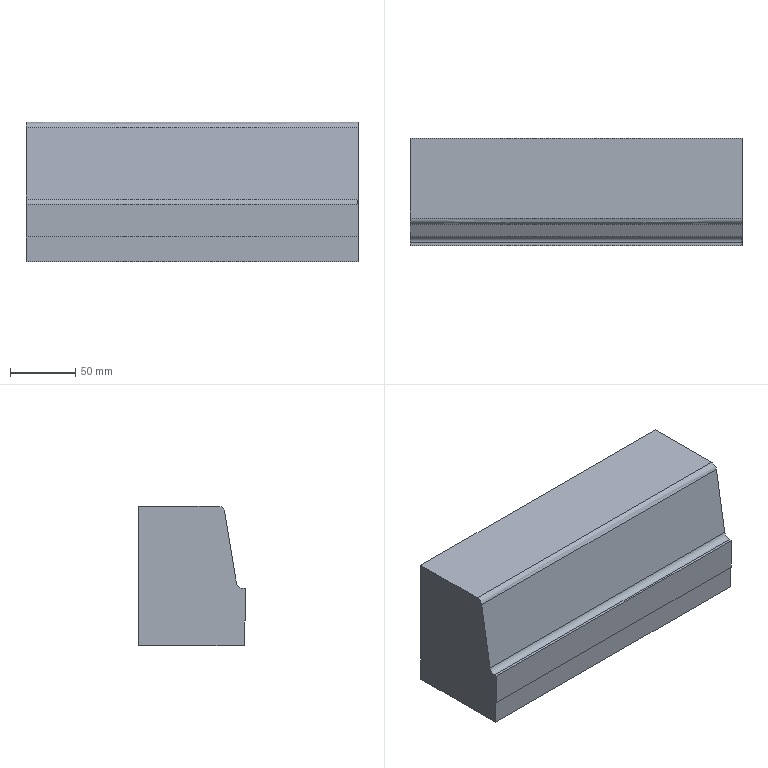Part | NX | features solid 2 | 1 solid | 22 faces | box 255 x 82.128 x 107.133 mm | volume 2023073 mm3 | plane 9 | cylinder 6 | spline 4 | cone 3 | commonest cylinder face diameters 12 x3 20 x2 10 x1
STEP:
#1=CARTESIAN_POINT('',(150.,175.,-20.));
#2=VERTEX_POINT('',#1);
#3=CARTESIAN_POINT('',(150.,175.,-30.));
#4=DIRECTION('',(0.,1.,0.));
#5=DIRECTION('',(0.,0.,1.));
#6=AXIS2_PLACEMENT_3D('',#3,#4,#5);
#7=CIRCLE('',#6,10.);
#8=EDGE_CURVE('',#2,#2,#7,.F.);
#9=ORIENTED_EDGE('',*,*,#8,.T.);
#10=EDGE_LOOP('',(#9));
#11=FACE_BOUND('',#10,.T.);
#12=CARTESIAN_POINT('',(-25.,175.,-20.));
#13=VERTEX_POINT('',#12);
#14=CARTESIAN_POINT('',(-25.,175.,-30.));
#15=DIRECTION('',(0.,1.,0.));
#16=DIRECTION('',(0.,0.,1.));
#17=AXIS2_PLACEMENT_3D('',#14,#15,#16);
#18=CIRCLE('',#17,10.);
#19=EDGE_CURVE('',#13,#13,#18,.F.);
#20=ORIENTED_EDGE('',*,*,#19,.T.);
#21=EDGE_LOOP('',(#20));
#22=FACE_BOUND('',#21,.T.);
#23=CARTESIAN_POINT('',(165.,175.,1.));
#24=VERTEX_POINT('',#23);
#25=CARTESIAN_POINT('',(165.,175.,-5.));
#26=DIRECTION('',(0.,1.,0.));
#27=DIRECTION('',(0.,0.,1.));
#28=AXIS2_PLACEMENT_3D('',#25,#26,#27);
#29=CIRCLE('',#28,6.);
#30=EDGE_CURVE('',#24,#24,#29,.F.);
#31=ORIENTED_EDGE('',*,*,#30,.T.);
#32=EDGE_LOOP('',(#31));
#33=FACE_BOUND('',#32,.T.);
#34=CARTESIAN_POINT('',(65.,175.,-24.));
#35=VERTEX_POINT('',#34);
#36=CARTESIAN_POINT('',(65.,175.,-30.));
#37=DIRECTION('',(0.,1.,0.));
#38=DIRECTION('',(0.,0.,1.));
#39=AXIS2_PLACEMENT_3D('',#36,#37,#38);
#40=CIRCLE('',#39,6.);
#41=EDGE_CURVE('',#35,#35,#40,.F.);
#42=ORIENTED_EDGE('',*,*,#41,.T.);
#43=EDGE_LOOP('',(#42));
#44=FACE_BOUND('',#43,.T.);
#45=CARTESIAN_POINT('',(-40.,175.,1.));
#46=VERTEX_POINT('',#45);
#47=CARTESIAN_POINT('',(-40.,175.,-5.));
#48=DIRECTION('',(0.,1.,0.));
#49=DIRECTION('',(0.,0.,1.));
#50=AXIS2_PLACEMENT_3D('',#47,#48,#49);
#51=CIRCLE('',#50,6.);
#52=EDGE_CURVE('',#46,#46,#51,.F.);
#53=ORIENTED_EDGE('',*,*,#52,.T.);
#54=EDGE_LOOP('',(#53));
#55=FACE_BOUND('',#54,.T.);
#56=CARTESIAN_POINT('',(190.,175.,57.133));
#57=VERTEX_POINT('',#56);
#58=CARTESIAN_POINT('',(190.,175.,-50.));
#59=VERTEX_POINT('',#58);
#60=CARTESIAN_POINT('',(190.,175.,-10.));
#61=DIRECTION('',(0.,0.,-1.));
#62=VECTOR('',#61,1000.);
#63=LINE('',#60,#62);
#64=EDGE_CURVE('',#57,#59,#63,.T.);
#65=ORIENTED_EDGE('',*,*,#64,.T.);
#66=CARTESIAN_POINT('',(-65.,175.,-50.));
#67=VERTEX_POINT('',#66);
#68=CARTESIAN_POINT('',(695.224,175.,-50.));
#69=DIRECTION('',(-1.,0.,0.));
#70=VECTOR('',#69,1000.);
#71=LINE('',#68,#70);
#72=EDGE_CURVE('',#59,#67,#71,.T.);
#73=ORIENTED_EDGE('',*,*,#72,.T.);
#74=CARTESIAN_POINT('',(-65.,175.,57.133));
#75=VERTEX_POINT('',#74);
#76=CARTESIAN_POINT('',(-65.,175.,0.));
#77=DIRECTION('',(0.,0.,1.));
#78=VECTOR('',#77,1000.);
#79=LINE('',#76,#78);
#80=EDGE_CURVE('',#67,#75,#79,.T.);
#81=ORIENTED_EDGE('',*,*,#80,.T.);
#82=CARTESIAN_POINT('',(750.,175.,57.133));
#83=DIRECTION('',(-1.,0.,0.));
#84=VECTOR('',#83,1000.);
#85=LINE('',#82,#84);
#86=EDGE_CURVE('',#57,#75,#85,.T.);
#87=ORIENTED_EDGE('',*,*,#86,.F.);
#88=EDGE_LOOP('',(#65,#73,#81,#87));
#89=FACE_BOUND('',#88,.T.);
#90=CARTESIAN_POINT('',(750.,175.,-10.));
#91=DIRECTION('',(0.,1.,0.));
#92=DIRECTION('',(0.,0.,1.));
#93=AXIS2_PLACEMENT_3D('',#90,#91,#92);
#94=PLANE('',#93);
#95=ADVANCED_FACE('',(#11,#22,#33,#44,#55,#89),#94,.T.);
#96=CARTESIAN_POINT('',(190.,108.917,52.95));
#97=VERTEX_POINT('',#96);
#98=CARTESIAN_POINT('',(-65.,108.917,52.95));
#99=VERTEX_POINT('',#98);
#100=CARTESIAN_POINT('',(190.,108.917,52.95));
#101=CARTESIAN_POINT('',(105.,108.917,52.95));
#102=CARTESIAN_POINT('',(20.,108.917,52.95));
#103=CARTESIAN_POINT('',(-65.,108.917,52.95));
#104=B_SPLINE_CURVE_WITH_KNOTS('',3,(#100,#101,#102,#103),.UNSPECIFIED.,.F.,.F.,(4,4),(0.1755,0.623),.UNSPECIFIED.);
#105=EDGE_CURVE('',#97,#99,#104,.T.);
#106=ORIENTED_EDGE('',*,*,#105,.F.);
#107=CARTESIAN_POINT('',(190.,113.85,57.133));
#108=VERTEX_POINT('',#107);
#109=CARTESIAN_POINT('',(190.,113.85,52.133));
#110=DIRECTION('',(1.,0.,0.));
#111=DIRECTION('',(0.,0.,-1.));
#112=AXIS2_PLACEMENT_3D('',#109,#110,#111);
#113=CIRCLE('',#112,5.);
#114=EDGE_CURVE('',#97,#108,#113,.F.);
#115=ORIENTED_EDGE('',*,*,#114,.T.);
#116=CARTESIAN_POINT('',(-65.,113.85,57.133));
#117=VERTEX_POINT('',#116);
#118=CARTESIAN_POINT('',(-65.,113.85,57.133));
#119=CARTESIAN_POINT('',(20.,113.85,57.133));
#120=CARTESIAN_POINT('',(105.,113.85,57.133));
#121=CARTESIAN_POINT('',(190.,113.85,57.133));
#122=B_SPLINE_CURVE_WITH_KNOTS('',3,(#118,#119,#120,#121),.UNSPECIFIED.,.F.,.F.,(4,4),(0.377,0.8245),.UNSPECIFIED.);
#123=EDGE_CURVE('',#117,#108,#122,.T.);
#124=ORIENTED_EDGE('',*,*,#123,.F.);
#125=CARTESIAN_POINT('',(-65.,113.85,52.133));
#126=DIRECTION('',(1.,0.,0.));
#127=DIRECTION('',(0.,0.,-1.));
#128=AXIS2_PLACEMENT_3D('',#125,#126,#127);
#129=CIRCLE('',#128,5.);
#130=EDGE_CURVE('',#99,#117,#129,.F.);
#131=ORIENTED_EDGE('',*,*,#130,.F.);
#132=EDGE_LOOP('',(#106,#115,#124,#131));
#133=FACE_BOUND('',#132,.T.);
#134=CARTESIAN_POINT('',(190.,113.85,57.133));
#135=CARTESIAN_POINT('',(190.,109.61,57.133));
#136=CARTESIAN_POINT('',(190.,108.917,52.95));
#137=CARTESIAN_POINT('',(105.,113.85,57.133));
#138=CARTESIAN_POINT('',(105.,109.61,57.133));
#139=CARTESIAN_POINT('',(105.,108.917,52.95));
#140=CARTESIAN_POINT('',(20.,113.85,57.133));
#141=CARTESIAN_POINT('',(20.,109.61,57.133));
#142=CARTESIAN_POINT('',(20.,108.917,52.95));
#143=CARTESIAN_POINT('',(-65.,113.85,57.133));
#144=CARTESIAN_POINT('',(-65.,109.61,57.133));
#145=CARTESIAN_POINT('',(-65.,108.917,52.95));
#146=(BOUNDED_SURFACE()B_SPLINE_SURFACE(3,2,((#134,#135,#136),(#137,#138,#139),(#140,#141,#142),(#143,#144,#145)),.UNSPECIFIED.,.F.,.F.,.F.)B_SPLINE_SURFACE_WITH_KNOTS((4,4),(3,3),(0.2812,0.5362),(0.,1.),.PIECEWISE_BEZIER_KNOTS.)GEOMETRIC_REPRESENTATION_ITEM()RATIONAL_B_SPLINE_SURFACE(((1.,0.7627,1.),(1.,0.7627,1.),(1.,0.7627,1.),(1.,0.7627,1.)))REPRESENTATION_ITEM('')SURFACE());
#147=ADVANCED_FACE('',(#133),#146,.T.);
#148=CARTESIAN_POINT('',(190.,99.848,-1.821));
#149=VERTEX_POINT('',#148);
#150=CARTESIAN_POINT('',(-65.,99.848,-1.821));
#151=VERTEX_POINT('',#150);
#152=CARTESIAN_POINT('',(190.,99.848,-1.821));
#153=CARTESIAN_POINT('',(105.,99.848,-1.821));
#154=CARTESIAN_POINT('',(20.,99.848,-1.821));
#155=CARTESIAN_POINT('',(-65.,99.848,-1.821));
#156=B_SPLINE_CURVE_WITH_KNOTS('',3,(#152,#153,#154,#155),.UNSPECIFIED.,.F.,.F.,(4,4),(0.1755,0.623),.UNSPECIFIED.);
#157=EDGE_CURVE('',#149,#151,#156,.T.);
#158=ORIENTED_EDGE('',*,*,#157,.F.);
#159=CARTESIAN_POINT('',(190.,104.878,28.559));
#160=DIRECTION('',(0.,0.1634,0.9866));
#161=VECTOR('',#160,1000.);
#162=LINE('',#159,#161);
#163=EDGE_CURVE('',#149,#97,#162,.T.);
#164=ORIENTED_EDGE('',*,*,#163,.T.);
#165=ORIENTED_EDGE('',*,*,#105,.T.);
#166=CARTESIAN_POINT('',(-65.,104.878,28.559));
#167=DIRECTION('',(0.,0.1634,0.9866));
#168=VECTOR('',#167,1000.);
#169=LINE('',#166,#168);
#170=EDGE_CURVE('',#151,#99,#169,.T.);
#171=ORIENTED_EDGE('',*,*,#170,.F.);
#172=EDGE_LOOP('',(#158,#164,#165,#171));
#173=FACE_BOUND('',#172,.T.);
#174=CARTESIAN_POINT('',(733.717,97.479,-16.126));
#175=CARTESIAN_POINT('',(-723.536,97.479,-16.126));
#176=CARTESIAN_POINT('',(733.717,112.278,73.243));
#177=CARTESIAN_POINT('',(-723.536,112.278,73.243));
#178=B_SPLINE_SURFACE_WITH_KNOTS('',1,1,((#174,#175),(#176,#177)),.PLANE_SURF.,.F.,.F.,.F.,(2,2),(2,2),(0.,1.902),(0.,1.),.UNSPECIFIED.);
#179=ADVANCED_FACE('',(#173),#178,.T.);
#180=CARTESIAN_POINT('',(190.,94.872,-6.004));
#181=VERTEX_POINT('',#180);
#182=CARTESIAN_POINT('',(190.,94.915,-1.004));
#183=DIRECTION('',(1.,0.,0.));
#184=DIRECTION('',(0.,0.,-1.));
#185=AXIS2_PLACEMENT_3D('',#182,#183,#184);
#186=CIRCLE('',#185,5.);
#187=EDGE_CURVE('',#149,#181,#186,.F.);
#188=ORIENTED_EDGE('',*,*,#187,.F.);
#189=ORIENTED_EDGE('',*,*,#157,.T.);
#190=CARTESIAN_POINT('',(-65.,94.872,-6.004));
#191=VERTEX_POINT('',#190);
#192=CARTESIAN_POINT('',(-65.,94.915,-1.004));
#193=DIRECTION('',(1.,0.,0.));
#194=DIRECTION('',(0.,0.,-1.));
#195=AXIS2_PLACEMENT_3D('',#192,#193,#194);
#196=CIRCLE('',#195,5.);
#197=EDGE_CURVE('',#151,#191,#196,.F.);
#198=ORIENTED_EDGE('',*,*,#197,.T.);
#199=CARTESIAN_POINT('',(-65.,94.872,-6.004));
#200=CARTESIAN_POINT('',(20.,94.872,-6.004));
#201=CARTESIAN_POINT('',(105.,94.872,-6.004));
#202=CARTESIAN_POINT('',(190.,94.872,-6.004));
#203=B_SPLINE_CURVE_WITH_KNOTS('',3,(#199,#200,#201,#202),.UNSPECIFIED.,.F.,.F.,(4,4),(0.377,0.8245),.UNSPECIFIED.);
#204=EDGE_CURVE('',#191,#181,#203,.T.);
#205=ORIENTED_EDGE('',*,*,#204,.T.);
#206=EDGE_LOOP('',(#188,#189,#198,#205));
#207=FACE_BOUND('',#206,.T.);
#208=CARTESIAN_POINT('',(6000290.,94.915,-1.004));
#209=DIRECTION('',(-1.,0.,0.));
#210=DIRECTION('',(0.,-0.1634,-0.9866));
#211=AXIS2_PLACEMENT_3D('',#208,#209,#210);
#212=CYLINDRICAL_SURFACE('',#211,5.);
#213=ADVANCED_FACE('',(#207),#212,.F.);
#214=CARTESIAN_POINT('',(190.,92.872,-5.987));
#215=VERTEX_POINT('',#214);
#216=CARTESIAN_POINT('',(190.,170.032,-6.646));
#217=DIRECTION('',(0.,-1.,0.008536));
#218=VECTOR('',#217,1000.);
#219=LINE('',#216,#218);
#220=EDGE_CURVE('',#181,#215,#219,.T.);
#221=ORIENTED_EDGE('',*,*,#220,.F.);
#222=ORIENTED_EDGE('',*,*,#204,.F.);
#223=CARTESIAN_POINT('',(-65.,92.872,-5.987));
#224=VERTEX_POINT('',#223);
#225=CARTESIAN_POINT('',(-65.,170.032,-6.646));
#226=DIRECTION('',(0.,-1.,0.008536));
#227=VECTOR('',#226,1000.);
#228=LINE('',#225,#227);
#229=EDGE_CURVE('',#191,#224,#228,.T.);
#230=ORIENTED_EDGE('',*,*,#229,.T.);
#231=CARTESIAN_POINT('',(290.,92.872,-5.987));
#232=DIRECTION('',(1.,0.,0.));
#233=VECTOR('',#232,1000.);
#234=LINE('',#231,#233);
#235=EDGE_CURVE('',#224,#215,#234,.T.);
#236=ORIENTED_EDGE('',*,*,#235,.T.);
#237=EDGE_LOOP('',(#221,#222,#230,#236));
#238=FACE_BOUND('',#237,.T.);
#239=CARTESIAN_POINT('',(120.529,170.032,-6.646));
#240=DIRECTION('',(0.,-0.008536,-1.));
#241=DIRECTION('',(0.,-1.,0.008536));
#242=AXIS2_PLACEMENT_3D('',#239,#240,#241);
#243=PLANE('',#242);
#244=ADVANCED_FACE('',(#238),#243,.F.);
#245=CARTESIAN_POINT('',(190.,92.872,-30.987));
#246=VERTEX_POINT('',#245);
#247=CARTESIAN_POINT('',(-65.,92.872,-30.987));
#248=VERTEX_POINT('',#247);
#249=CARTESIAN_POINT('',(190.,92.872,-30.987));
#250=CARTESIAN_POINT('',(105.,92.872,-30.987));
#251=CARTESIAN_POINT('',(20.,92.872,-30.987));
#252=CARTESIAN_POINT('',(-65.,92.872,-30.987));
#253=B_SPLINE_CURVE_WITH_KNOTS('',3,(#249,#250,#251,#252),.UNSPECIFIED.,.F.,.F.,(4,4),(0.1,0.355),.UNSPECIFIED.);
#254=EDGE_CURVE('',#246,#248,#253,.T.);
#255=ORIENTED_EDGE('',*,*,#254,.F.);
#256=CARTESIAN_POINT('',(190.,92.872,200.));
#257=DIRECTION('',(0.,0.,1.));
#258=VECTOR('',#257,1000.);
#259=LINE('',#256,#258);
#260=EDGE_CURVE('',#246,#215,#259,.T.);
#261=ORIENTED_EDGE('',*,*,#260,.T.);
#262=ORIENTED_EDGE('',*,*,#235,.F.);
#263=CARTESIAN_POINT('',(-65.,92.872,200.));
#264=DIRECTION('',(0.,0.,1.));
#265=VECTOR('',#264,1000.);
#266=LINE('',#263,#265);
#267=EDGE_CURVE('',#248,#224,#266,.T.);
#268=ORIENTED_EDGE('',*,*,#267,.F.);
#269=EDGE_LOOP('',(#255,#261,#262,#268));
#270=FACE_BOUND('',#269,.T.);
#271=CARTESIAN_POINT('',(290.,92.872,200.));
#272=DIRECTION('',(0.,-1.,0.));
#273=DIRECTION('',(1.,0.,0.));
#274=AXIS2_PLACEMENT_3D('',#271,#272,#273);
#275=PLANE('',#274);
#276=ADVANCED_FACE('',(#270),#275,.T.);
#277=CARTESIAN_POINT('',(-65.,93.872,-30.987));
#278=VERTEX_POINT('',#277);
#279=CARTESIAN_POINT('',(-65.,92.872,-30.987));
#280=CARTESIAN_POINT('',(-65.,93.206,-30.987));
#281=CARTESIAN_POINT('',(-65.,93.539,-30.987));
#282=CARTESIAN_POINT('',(-65.,93.872,-30.987));
#283=B_SPLINE_CURVE_WITH_KNOTS('',3,(#279,#280,#281,#282),.UNSPECIFIED.,.F.,.F.,(4,4),(0.0003492,0.001349),.UNSPECIFIED.);
#284=EDGE_CURVE('',#248,#278,#283,.T.);
#285=ORIENTED_EDGE('',*,*,#284,.T.);
#286=CARTESIAN_POINT('',(190.,93.889,-30.987));
#287=VERTEX_POINT('',#286);
#288=CARTESIAN_POINT('',(190.,93.889,-30.987));
#289=CARTESIAN_POINT('',(105.,93.866,-30.987));
#290=CARTESIAN_POINT('',(20.,93.872,-30.987));
#291=CARTESIAN_POINT('',(-65.,93.872,-30.987));
#292=B_SPLINE_CURVE_WITH_KNOTS('',3,(#288,#289,#290,#291),.UNSPECIFIED.,.F.,.F.,(4,4),(0.1333,0.3889),.UNSPECIFIED.);
#293=EDGE_CURVE('',#278,#287,#292,.F.);
#294=ORIENTED_EDGE('',*,*,#293,.T.);
#295=CARTESIAN_POINT('',(190.,92.872,-30.987));
#296=CARTESIAN_POINT('',(190.,93.211,-30.987));
#297=CARTESIAN_POINT('',(190.,93.55,-30.987));
#298=CARTESIAN_POINT('',(190.,93.889,-30.987));
#299=B_SPLINE_CURVE_WITH_KNOTS('',3,(#295,#296,#297,#298),.UNSPECIFIED.,.F.,.F.,(4,4),(0.0003325,0.001349),.UNSPECIFIED.);
#300=EDGE_CURVE('',#246,#287,#299,.T.);
#301=ORIENTED_EDGE('',*,*,#300,.F.);
#302=ORIENTED_EDGE('',*,*,#254,.T.);
#303=EDGE_LOOP('',(#285,#294,#301,#302));
#304=FACE_BOUND('',#303,.T.);
#305=CARTESIAN_POINT('',(-65.,93.872,-30.987));
#306=CARTESIAN_POINT('',(-41.607,93.872,-30.987));
#307=CARTESIAN_POINT('',(-18.213,93.872,-30.987));
#308=CARTESIAN_POINT('',(52.65,93.872,-30.987));
#309=CARTESIAN_POINT('',(100.12,93.872,-30.987));
#310=CARTESIAN_POINT('',(162.237,93.882,-30.987));
#311=CARTESIAN_POINT('',(176.884,93.885,-30.987));
#312=CARTESIAN_POINT('',(191.53,93.889,-30.987));
#313=CARTESIAN_POINT('',(-65.,92.849,-30.987));
#314=CARTESIAN_POINT('',(-41.607,92.849,-30.987));
#315=CARTESIAN_POINT('',(-18.213,92.849,-30.987));
#316=CARTESIAN_POINT('',(52.65,92.849,-30.987));
#317=CARTESIAN_POINT('',(100.12,92.849,-30.987));
#318=CARTESIAN_POINT('',(162.237,92.859,-30.987));
#319=CARTESIAN_POINT('',(176.884,92.863,-30.987));
#320=CARTESIAN_POINT('',(191.53,92.867,-30.987));
#321=B_SPLINE_SURFACE_WITH_KNOTS('',1,3,((#305,#306,#307,#308,#309,#310,#311,#312),(#313,#314,#315,#316,#317,#318,#319,#320)),.RULED_SURF.,.F.,.F.,.F.,(2,2),(4,2,2,4),(0.4,0.5023),(0.6129,0.6894,0.8447,0.8926),.UNSPECIFIED.);
#322=ADVANCED_FACE('',(#304),#321,.F.);
#323=ORIENTED_EDGE('',*,*,#293,.F.);
#324=CARTESIAN_POINT('',(-65.,93.872,-50.));
#325=VERTEX_POINT('',#324);
#326=CARTESIAN_POINT('',(-65.,93.872,-50.));
#327=DIRECTION('',(0.,0.,-1.));
#328=VECTOR('',#327,1000.);
#329=LINE('',#326,#328);
#330=EDGE_CURVE('',#325,#278,#329,.F.);
#331=ORIENTED_EDGE('',*,*,#330,.F.);
#332=CARTESIAN_POINT('',(190.,93.889,-50.));
#333=VERTEX_POINT('',#332);
#334=CARTESIAN_POINT('',(190.,93.889,-50.));
#335=CARTESIAN_POINT('',(105.,93.866,-50.));
#336=CARTESIAN_POINT('',(20.,93.872,-50.));
#337=CARTESIAN_POINT('',(-65.,93.872,-50.));
#338=B_SPLINE_CURVE_WITH_KNOTS('',3,(#334,#335,#336,#337),.UNSPECIFIED.,.F.,.F.,(4,4),(0.7975,1.053),.UNSPECIFIED.);
#339=EDGE_CURVE('',#333,#325,#338,.T.);
#340=ORIENTED_EDGE('',*,*,#339,.F.);
#341=CARTESIAN_POINT('',(190.,93.889,-40.494));
#342=DIRECTION('',(0.,0.,-1.));
#343=VECTOR('',#342,1000.);
#344=LINE('',#341,#343);
#345=EDGE_CURVE('',#287,#333,#344,.T.);
#346=ORIENTED_EDGE('',*,*,#345,.F.);
#347=EDGE_LOOP('',(#323,#331,#340,#346));
#348=FACE_BOUND('',#347,.T.);
#349=CARTESIAN_POINT('',(-65.,93.872,-30.987));
#350=CARTESIAN_POINT('',(-65.,93.872,-50.114));
#351=CARTESIAN_POINT('',(19.999,93.872,-30.987));
#352=CARTESIAN_POINT('',(19.999,93.872,-50.114));
#353=CARTESIAN_POINT('',(104.998,93.866,-30.987));
#354=CARTESIAN_POINT('',(104.998,93.866,-50.114));
#355=CARTESIAN_POINT('',(190.,93.889,-30.987));
#356=CARTESIAN_POINT('',(190.,93.889,-50.114));
#357=B_SPLINE_SURFACE_WITH_KNOTS('',3,1,((#349,#350),(#351,#352),(#353,#354),(#355,#356)),.SURF_OF_LINEAR_EXTRUSION.,.F.,.F.,.F.,(4,4),(2,2),(0.6129,0.891),(0.,1.),.PIECEWISE_BEZIER_KNOTS.);
#358=ADVANCED_FACE('',(#348),#357,.F.);
#359=ORIENTED_EDGE('',*,*,#300,.T.);
#360=ORIENTED_EDGE('',*,*,#345,.T.);
#361=CARTESIAN_POINT('',(190.,82.819,-50.));
#362=DIRECTION('',(0.,1.,0.));
#363=VECTOR('',#362,1000.);
#364=LINE('',#361,#363);
#365=EDGE_CURVE('',#333,#59,#364,.T.);
#366=ORIENTED_EDGE('',*,*,#365,.T.);
#367=ORIENTED_EDGE('',*,*,#64,.F.);
#368=CARTESIAN_POINT('',(190.,109.61,57.133));
#369=DIRECTION('',(0.,-1.,0.));
#370=VECTOR('',#369,1000.);
#371=LINE('',#368,#370);
#372=EDGE_CURVE('',#57,#108,#371,.T.);
#373=ORIENTED_EDGE('',*,*,#372,.T.);
#374=ORIENTED_EDGE('',*,*,#114,.F.);
#375=ORIENTED_EDGE('',*,*,#163,.F.);
#376=ORIENTED_EDGE('',*,*,#187,.T.);
#377=ORIENTED_EDGE('',*,*,#220,.T.);
#378=ORIENTED_EDGE('',*,*,#260,.F.);
#379=EDGE_LOOP('',(#359,#360,#366,#367,#373,#374,#375,#376,#377,#378));
#380=FACE_BOUND('',#379,.T.);
#381=CARTESIAN_POINT('',(190.,-361.,0.));
#382=DIRECTION('',(1.,0.,0.));
#383=DIRECTION('',(0.,0.,-1.));
#384=AXIS2_PLACEMENT_3D('',#381,#382,#383);
#385=PLANE('',#384);
#386=ADVANCED_FACE('',(#380),#385,.T.);
#387=ORIENTED_EDGE('',*,*,#372,.F.);
#388=ORIENTED_EDGE('',*,*,#86,.T.);
#389=CARTESIAN_POINT('',(-65.,109.61,57.133));
#390=DIRECTION('',(0.,-1.,0.));
#391=VECTOR('',#390,1000.);
#392=LINE('',#389,#391);
#393=EDGE_CURVE('',#75,#117,#392,.T.);
#394=ORIENTED_EDGE('',*,*,#393,.T.);
#395=ORIENTED_EDGE('',*,*,#123,.T.);
#396=EDGE_LOOP('',(#387,#388,#394,#395));
#397=FACE_BOUND('',#396,.T.);
#398=CARTESIAN_POINT('',(290.,109.61,57.133));
#399=DIRECTION('',(0.,0.,-1.));
#400=DIRECTION('',(-1.,0.,0.));
#401=AXIS2_PLACEMENT_3D('',#398,#399,#400);
#402=PLANE('',#401);
#403=ADVANCED_FACE('',(#397),#402,.F.);
#404=ORIENTED_EDGE('',*,*,#330,.T.);
#405=ORIENTED_EDGE('',*,*,#284,.F.);
#406=ORIENTED_EDGE('',*,*,#267,.T.);
#407=ORIENTED_EDGE('',*,*,#229,.F.);
#408=ORIENTED_EDGE('',*,*,#197,.F.);
#409=ORIENTED_EDGE('',*,*,#170,.T.);
#410=ORIENTED_EDGE('',*,*,#130,.T.);
#411=ORIENTED_EDGE('',*,*,#393,.F.);
#412=ORIENTED_EDGE('',*,*,#80,.F.);
#413=CARTESIAN_POINT('',(-65.,-361.,-50.));
#414=DIRECTION('',(0.,-1.,0.));
#415=VECTOR('',#414,1000.);
#416=LINE('',#413,#415);
#417=EDGE_CURVE('',#325,#67,#416,.F.);
#418=ORIENTED_EDGE('',*,*,#417,.F.);
#419=EDGE_LOOP('',(#404,#405,#406,#407,#408,#409,#410,#411,#412,#418));
#420=FACE_BOUND('',#419,.T.);
#421=CARTESIAN_POINT('',(-65.,-361.,0.));
#422=DIRECTION('',(1.,0.,0.));
#423=DIRECTION('',(0.,0.,-1.));
#424=AXIS2_PLACEMENT_3D('',#421,#422,#423);
#425=PLANE('',#424);
#426=ADVANCED_FACE('',(#420),#425,.F.);
#427=ORIENTED_EDGE('',*,*,#72,.F.);
#428=ORIENTED_EDGE('',*,*,#365,.F.);
#429=ORIENTED_EDGE('',*,*,#339,.T.);
#430=ORIENTED_EDGE('',*,*,#417,.T.);
#431=EDGE_LOOP('',(#427,#428,#429,#430));
#432=FACE_BOUND('',#431,.T.);
#433=CARTESIAN_POINT('',(695.224,82.819,-50.));
#434=DIRECTION('',(0.,0.,1.));
#435=DIRECTION('',(1.,0.,0.));
#436=AXIS2_PLACEMENT_3D('',#433,#434,#435);
#437=PLANE('',#436);
#438=ADVANCED_FACE('',(#432),#437,.F.);
#439=CARTESIAN_POINT('',(-40.,144.,-11.));
#440=VERTEX_POINT('',#439);
#441=CARTESIAN_POINT('',(-40.,144.,-5.));
#442=DIRECTION('',(0.,-1.,0.));
#443=DIRECTION('',(0.,0.,-1.));
#444=AXIS2_PLACEMENT_3D('',#441,#442,#443);
#445=CIRCLE('',#444,6.);
#446=EDGE_CURVE('',#440,#440,#445,.T.);
#447=ORIENTED_EDGE('',*,*,#446,.F.);
#448=EDGE_LOOP('',(#447));
#449=FACE_BOUND('',#448,.T.);
#450=CARTESIAN_POINT('',(-40.,140.395,-5.));
#451=VERTEX_POINT('',#450);
#452=VERTEX_LOOP('',#451);
#453=FACE_BOUND('',#452,.T.);
#454=CARTESIAN_POINT('',(-40.,144.,-5.));
#455=DIRECTION('',(0.,1.,0.));
#456=DIRECTION('',(0.,0.,1.));
#457=AXIS2_PLACEMENT_3D('',#454,#455,#456);
#458=CONICAL_SURFACE('',#457,6.,1.03);
#459=ADVANCED_FACE('',(#449,#453),#458,.F.);
#460=ORIENTED_EDGE('',*,*,#446,.T.);
#461=EDGE_LOOP('',(#460));
#462=FACE_BOUND('',#461,.T.);
#463=ORIENTED_EDGE('',*,*,#52,.F.);
#464=EDGE_LOOP('',(#463));
#465=FACE_BOUND('',#464,.T.);
#466=CARTESIAN_POINT('',(-40.,174.,-5.));
#467=DIRECTION('',(0.,-1.,0.));
#468=DIRECTION('',(0.,0.,-1.));
#469=AXIS2_PLACEMENT_3D('',#466,#467,#468);
#470=CYLINDRICAL_SURFACE('',#469,6.);
#471=ADVANCED_FACE('',(#462,#465),#470,.F.);
#472=CARTESIAN_POINT('',(65.,144.,-36.));
#473=VERTEX_POINT('',#472);
#474=CARTESIAN_POINT('',(65.,144.,-30.));
#475=DIRECTION('',(0.,-1.,0.));
#476=DIRECTION('',(0.,0.,-1.));
#477=AXIS2_PLACEMENT_3D('',#474,#475,#476);
#478=CIRCLE('',#477,6.);
#479=EDGE_CURVE('',#473,#473,#478,.T.);
#480=ORIENTED_EDGE('',*,*,#479,.F.);
#481=EDGE_LOOP('',(#480));
#482=FACE_BOUND('',#481,.T.);
#483=CARTESIAN_POINT('',(65.,140.395,-30.));
#484=VERTEX_POINT('',#483);
#485=VERTEX_LOOP('',#484);
#486=FACE_BOUND('',#485,.T.);
#487=CARTESIAN_POINT('',(65.,144.,-30.));
#488=DIRECTION('',(0.,1.,0.));
#489=DIRECTION('',(0.,0.,1.));
#490=AXIS2_PLACEMENT_3D('',#487,#488,#489);
#491=CONICAL_SURFACE('',#490,6.,1.03);
#492=ADVANCED_FACE('',(#482,#486),#491,.F.);
#493=ORIENTED_EDGE('',*,*,#479,.T.);
#494=EDGE_LOOP('',(#493));
#495=FACE_BOUND('',#494,.T.);
#496=ORIENTED_EDGE('',*,*,#41,.F.);
#497=EDGE_LOOP('',(#496));
#498=FACE_BOUND('',#497,.T.);
#499=CARTESIAN_POINT('',(65.,174.,-30.));
#500=DIRECTION('',(0.,-1.,0.));
#501=DIRECTION('',(0.,0.,-1.));
#502=AXIS2_PLACEMENT_3D('',#499,#500,#501);
#503=CYLINDRICAL_SURFACE('',#502,6.);
#504=ADVANCED_FACE('',(#495,#498),#503,.F.);
#505=CARTESIAN_POINT('',(165.,144.,-11.));
#506=VERTEX_POINT('',#505);
#507=CARTESIAN_POINT('',(165.,144.,-5.));
#508=DIRECTION('',(0.,-1.,0.));
#509=DIRECTION('',(0.,0.,-1.));
#510=AXIS2_PLACEMENT_3D('',#507,#508,#509);
#511=CIRCLE('',#510,6.);
#512=EDGE_CURVE('',#506,#506,#511,.T.);
#513=ORIENTED_EDGE('',*,*,#512,.F.);
#514=EDGE_LOOP('',(#513));
#515=FACE_BOUND('',#514,.T.);
#516=CARTESIAN_POINT('',(165.,140.395,-5.));
#517=VERTEX_POINT('',#516);
#518=VERTEX_LOOP('',#517);
#519=FACE_BOUND('',#518,.T.);
#520=CARTESIAN_POINT('',(165.,144.,-5.));
#521=DIRECTION('',(0.,1.,0.));
#522=DIRECTION('',(0.,0.,1.));
#523=AXIS2_PLACEMENT_3D('',#520,#521,#522);
#524=CONICAL_SURFACE('',#523,6.,1.03);
#525=ADVANCED_FACE('',(#515,#519),#524,.F.);
#526=ORIENTED_EDGE('',*,*,#512,.T.);
#527=EDGE_LOOP('',(#526));
#528=FACE_BOUND('',#527,.T.);
#529=ORIENTED_EDGE('',*,*,#30,.F.);
#530=EDGE_LOOP('',(#529));
#531=FACE_BOUND('',#530,.T.);
#532=CARTESIAN_POINT('',(165.,174.,-5.));
#533=DIRECTION('',(0.,-1.,0.));
#534=DIRECTION('',(0.,0.,-1.));
#535=AXIS2_PLACEMENT_3D('',#532,#533,#534);
#536=CYLINDRICAL_SURFACE('',#535,6.);
#537=ADVANCED_FACE('',(#528,#531),#536,.F.);
#538=CARTESIAN_POINT('',(-25.,144.,-40.));
#539=VERTEX_POINT('',#538);
#540=CARTESIAN_POINT('',(-25.,144.,-30.));
#541=DIRECTION('',(0.,-1.,0.));
#542=DIRECTION('',(0.,0.,-1.));
#543=AXIS2_PLACEMENT_3D('',#540,#541,#542);
#544=CIRCLE('',#543,10.);
#545=EDGE_CURVE('',#539,#539,#544,.T.);
#546=ORIENTED_EDGE('',*,*,#545,.T.);
#547=EDGE_LOOP('',(#546));
#548=FACE_BOUND('',#547,.T.);
#549=ORIENTED_EDGE('',*,*,#19,.F.);
#550=EDGE_LOOP('',(#549));
#551=FACE_BOUND('',#550,.T.);
#552=CARTESIAN_POINT('',(-25.,174.,-30.));
#553=DIRECTION('',(0.,-1.,0.));
#554=DIRECTION('',(0.,0.,-1.));
#555=AXIS2_PLACEMENT_3D('',#552,#553,#554);
#556=CYLINDRICAL_SURFACE('',#555,10.);
#557=ADVANCED_FACE('',(#548,#551),#556,.F.);
#558=ORIENTED_EDGE('',*,*,#545,.F.);
#559=EDGE_LOOP('',(#558));
#560=FACE_BOUND('',#559,.T.);
#561=CARTESIAN_POINT('',(-25.,144.,-30.));
#562=DIRECTION('',(0.,-1.,0.));
#563=DIRECTION('',(0.,0.,-1.));
#564=AXIS2_PLACEMENT_3D('',#561,#562,#563);
#565=PLANE('',#564);
#566=ADVANCED_FACE('',(#560),#565,.F.);
#567=CARTESIAN_POINT('',(150.,144.,-40.));
#568=VERTEX_POINT('',#567);
#569=CARTESIAN_POINT('',(150.,144.,-30.));
#570=DIRECTION('',(0.,-1.,0.));
#571=DIRECTION('',(0.,0.,-1.));
#572=AXIS2_PLACEMENT_3D('',#569,#570,#571);
#573=CIRCLE('',#572,10.);
#574=EDGE_CURVE('',#568,#568,#573,.T.);
#575=ORIENTED_EDGE('',*,*,#574,.T.);
#576=EDGE_LOOP('',(#575));
#577=FACE_BOUND('',#576,.T.);
#578=ORIENTED_EDGE('',*,*,#8,.F.);
#579=EDGE_LOOP('',(#578));
#580=FACE_BOUND('',#579,.T.);
#581=CARTESIAN_POINT('',(150.,174.,-30.));
#582=DIRECTION('',(0.,-1.,0.));
#583=DIRECTION('',(0.,0.,-1.));
#584=AXIS2_PLACEMENT_3D('',#581,#582,#583);
#585=CYLINDRICAL_SURFACE('',#584,10.);
#586=ADVANCED_FACE('',(#577,#580),#585,.F.);
#587=ORIENTED_EDGE('',*,*,#574,.F.);
#588=EDGE_LOOP('',(#587));
#589=FACE_BOUND('',#588,.T.);
#590=CARTESIAN_POINT('',(150.,144.,-30.));
#591=DIRECTION('',(0.,-1.,0.));
#592=DIRECTION('',(0.,0.,-1.));
#593=AXIS2_PLACEMENT_3D('',#590,#591,#592);
#594=PLANE('',#593);
#595=ADVANCED_FACE('',(#589),#594,.F.);
#596=CLOSED_SHELL('',(#95,#147,#179,#213,#244,#276,#322,#358,#386,#403,#426,#438,#459,#471,#492,#504,#525,#537,#557,#566,#586,#595));
#597=MANIFOLD_SOLID_BREP('',#596);
#598=(LENGTH_UNIT()NAMED_UNIT(*)SI_UNIT(.MILLI.,.METRE.));
#599=UNCERTAINTY_MEASURE_WITH_UNIT(LENGTH_MEASURE(0.0508),#598,'','');
#600=(NAMED_UNIT(*)PLANE_ANGLE_UNIT()SI_UNIT($,.RADIAN.));
#601=(NAMED_UNIT(*)SI_UNIT($,.STERADIAN.)SOLID_ANGLE_UNIT());
#602=(GEOMETRIC_REPRESENTATION_CONTEXT(3)GLOBAL_UNCERTAINTY_ASSIGNED_CONTEXT((#599))GLOBAL_UNIT_ASSIGNED_CONTEXT((#598,#600,#601))REPRESENTATION_CONTEXT('',''));
#603=ADVANCED_BREP_SHAPE_REPRESENTATION('',(#597),#602);